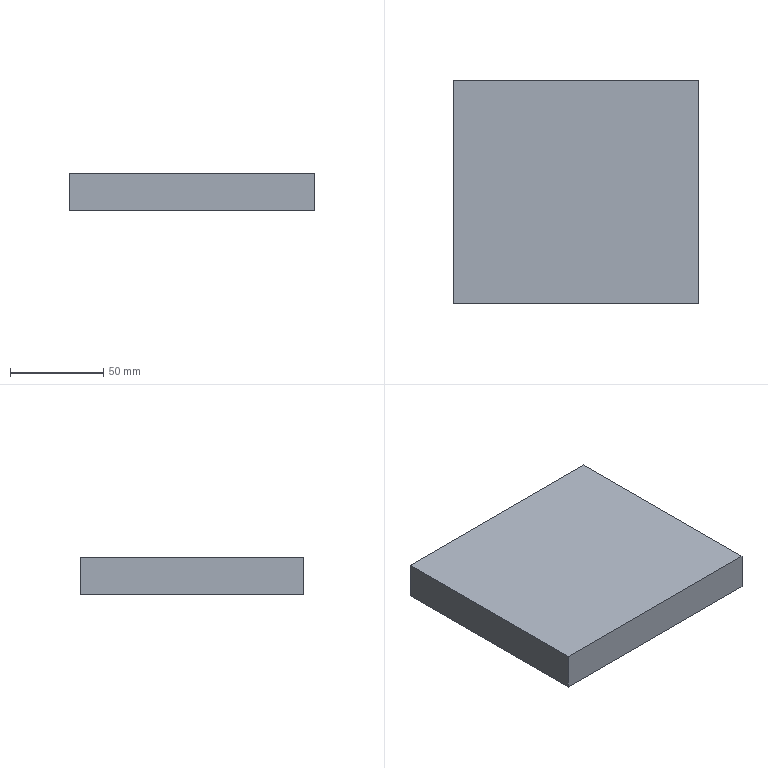Part | SolidWorks | features Extrusion 1 | 1 solid | 6 faces | box 132 x 120 x 20 mm | volume 316800 mm3 | plane 6
STEP:
#1=CARTESIAN_POINT('',(0.,120.,0.));
#2=VERTEX_POINT('',#1);
#3=CARTESIAN_POINT('',(0.,0.,0.));
#4=VERTEX_POINT('',#3);
#5=CARTESIAN_POINT('',(0.,0.,0.));
#6=DIRECTION('',(0.,-1.,0.));
#7=VECTOR('',#6,1000.);
#8=LINE('',#5,#7);
#9=EDGE_CURVE('',#2,#4,#8,.T.);
#10=ORIENTED_EDGE('',*,*,#9,.T.);
#11=CARTESIAN_POINT('',(0.,0.,20.));
#12=VERTEX_POINT('',#11);
#13=CARTESIAN_POINT('',(0.,0.,20.));
#14=DIRECTION('',(0.,0.,-1.));
#15=VECTOR('',#14,1000.);
#16=LINE('',#13,#15);
#17=EDGE_CURVE('',#12,#4,#16,.T.);
#18=ORIENTED_EDGE('',*,*,#17,.F.);
#19=CARTESIAN_POINT('',(0.,120.,20.));
#20=VERTEX_POINT('',#19);
#21=CARTESIAN_POINT('',(0.,0.,20.));
#22=DIRECTION('',(0.,-1.,0.));
#23=VECTOR('',#22,1000.);
#24=LINE('',#21,#23);
#25=EDGE_CURVE('',#20,#12,#24,.T.);
#26=ORIENTED_EDGE('',*,*,#25,.F.);
#27=CARTESIAN_POINT('',(0.,120.,20.));
#28=DIRECTION('',(0.,0.,-1.));
#29=VECTOR('',#28,1000.);
#30=LINE('',#27,#29);
#31=EDGE_CURVE('',#20,#2,#30,.T.);
#32=ORIENTED_EDGE('',*,*,#31,.T.);
#33=EDGE_LOOP('',(#10,#18,#26,#32));
#34=FACE_OUTER_BOUND('',#33,.T.);
#35=CARTESIAN_POINT('',(0.,0.,20.));
#36=DIRECTION('',(1.,0.,0.));
#37=DIRECTION('',(0.,0.,-1.));
#38=AXIS2_PLACEMENT_3D('',#35,#36,#37);
#39=PLANE('',#38);
#40=ADVANCED_FACE('',(#34),#39,.F.);
#41=CARTESIAN_POINT('',(132.,0.,0.));
#42=VERTEX_POINT('',#41);
#43=CARTESIAN_POINT('',(0.,0.,0.));
#44=DIRECTION('',(1.,0.,0.));
#45=VECTOR('',#44,1000.);
#46=LINE('',#43,#45);
#47=EDGE_CURVE('',#4,#42,#46,.T.);
#48=ORIENTED_EDGE('',*,*,#47,.T.);
#49=CARTESIAN_POINT('',(132.,0.,20.));
#50=VERTEX_POINT('',#49);
#51=CARTESIAN_POINT('',(132.,0.,20.));
#52=DIRECTION('',(0.,0.,-1.));
#53=VECTOR('',#52,1000.);
#54=LINE('',#51,#53);
#55=EDGE_CURVE('',#50,#42,#54,.T.);
#56=ORIENTED_EDGE('',*,*,#55,.F.);
#57=CARTESIAN_POINT('',(0.,0.,20.));
#58=DIRECTION('',(1.,0.,0.));
#59=VECTOR('',#58,1000.);
#60=LINE('',#57,#59);
#61=EDGE_CURVE('',#12,#50,#60,.T.);
#62=ORIENTED_EDGE('',*,*,#61,.F.);
#63=ORIENTED_EDGE('',*,*,#17,.T.);
#64=EDGE_LOOP('',(#48,#56,#62,#63));
#65=FACE_OUTER_BOUND('',#64,.T.);
#66=CARTESIAN_POINT('',(0.,0.,20.));
#67=DIRECTION('',(0.,1.,0.));
#68=DIRECTION('',(0.,0.,1.));
#69=AXIS2_PLACEMENT_3D('',#66,#67,#68);
#70=PLANE('',#69);
#71=ADVANCED_FACE('',(#65),#70,.F.);
#72=CARTESIAN_POINT('',(132.,120.,0.));
#73=VERTEX_POINT('',#72);
#74=CARTESIAN_POINT('',(132.,0.,0.));
#75=DIRECTION('',(0.,1.,0.));
#76=VECTOR('',#75,1000.);
#77=LINE('',#74,#76);
#78=EDGE_CURVE('',#42,#73,#77,.T.);
#79=ORIENTED_EDGE('',*,*,#78,.T.);
#80=CARTESIAN_POINT('',(132.,120.,20.));
#81=VERTEX_POINT('',#80);
#82=CARTESIAN_POINT('',(132.,120.,20.));
#83=DIRECTION('',(0.,0.,-1.));
#84=VECTOR('',#83,1000.);
#85=LINE('',#82,#84);
#86=EDGE_CURVE('',#81,#73,#85,.T.);
#87=ORIENTED_EDGE('',*,*,#86,.F.);
#88=CARTESIAN_POINT('',(132.,0.,20.));
#89=DIRECTION('',(0.,1.,0.));
#90=VECTOR('',#89,1000.);
#91=LINE('',#88,#90);
#92=EDGE_CURVE('',#50,#81,#91,.T.);
#93=ORIENTED_EDGE('',*,*,#92,.F.);
#94=ORIENTED_EDGE('',*,*,#55,.T.);
#95=EDGE_LOOP('',(#79,#87,#93,#94));
#96=FACE_OUTER_BOUND('',#95,.T.);
#97=CARTESIAN_POINT('',(132.,0.,20.));
#98=DIRECTION('',(-1.,0.,0.));
#99=DIRECTION('',(0.,0.,1.));
#100=AXIS2_PLACEMENT_3D('',#97,#98,#99);
#101=PLANE('',#100);
#102=ADVANCED_FACE('',(#96),#101,.F.);
#103=CARTESIAN_POINT('',(0.,120.,0.));
#104=DIRECTION('',(-1.,0.,0.));
#105=VECTOR('',#104,1000.);
#106=LINE('',#103,#105);
#107=EDGE_CURVE('',#73,#2,#106,.T.);
#108=ORIENTED_EDGE('',*,*,#107,.T.);
#109=ORIENTED_EDGE('',*,*,#31,.F.);
#110=CARTESIAN_POINT('',(0.,120.,20.));
#111=DIRECTION('',(-1.,0.,0.));
#112=VECTOR('',#111,1000.);
#113=LINE('',#110,#112);
#114=EDGE_CURVE('',#81,#20,#113,.T.);
#115=ORIENTED_EDGE('',*,*,#114,.F.);
#116=ORIENTED_EDGE('',*,*,#86,.T.);
#117=EDGE_LOOP('',(#108,#109,#115,#116));
#118=FACE_OUTER_BOUND('',#117,.T.);
#119=CARTESIAN_POINT('',(0.,120.,20.));
#120=DIRECTION('',(0.,-1.,0.));
#121=DIRECTION('',(0.,0.,-1.));
#122=AXIS2_PLACEMENT_3D('',#119,#120,#121);
#123=PLANE('',#122);
#124=ADVANCED_FACE('',(#118),#123,.F.);
#125=ORIENTED_EDGE('',*,*,#25,.T.);
#126=ORIENTED_EDGE('',*,*,#61,.T.);
#127=ORIENTED_EDGE('',*,*,#92,.T.);
#128=ORIENTED_EDGE('',*,*,#114,.T.);
#129=EDGE_LOOP('',(#125,#126,#127,#128));
#130=FACE_OUTER_BOUND('',#129,.T.);
#131=CARTESIAN_POINT('',(0.,0.,20.));
#132=DIRECTION('',(0.,0.,-1.));
#133=DIRECTION('',(-1.,0.,0.));
#134=AXIS2_PLACEMENT_3D('',#131,#132,#133);
#135=PLANE('',#134);
#136=ADVANCED_FACE('',(#130),#135,.F.);
#137=ORIENTED_EDGE('',*,*,#9,.F.);
#138=ORIENTED_EDGE('',*,*,#107,.F.);
#139=ORIENTED_EDGE('',*,*,#78,.F.);
#140=ORIENTED_EDGE('',*,*,#47,.F.);
#141=EDGE_LOOP('',(#137,#138,#139,#140));
#142=FACE_OUTER_BOUND('',#141,.T.);
#143=CARTESIAN_POINT('',(0.,0.,0.));
#144=DIRECTION('',(0.,0.,-1.));
#145=DIRECTION('',(-1.,0.,0.));
#146=AXIS2_PLACEMENT_3D('',#143,#144,#145);
#147=PLANE('',#146);
#148=ADVANCED_FACE('',(#142),#147,.T.);
#149=CLOSED_SHELL('',(#40,#71,#102,#124,#136,#148));
#150=MANIFOLD_SOLID_BREP('',#149);
#151=CARTESIAN_POINT('',(0.,0.,0.));
#152=DIRECTION('',(0.,0.,1.));
#153=DIRECTION('',(1.,0.,0.));
#154=AXIS2_PLACEMENT_3D('',#151,#152,#153);
#155=(LENGTH_UNIT()NAMED_UNIT(*)SI_UNIT(.MILLI.,.METRE.));
#156=UNCERTAINTY_MEASURE_WITH_UNIT(LENGTH_MEASURE(0.00001),#155,'','');
#157=(NAMED_UNIT(*)PLANE_ANGLE_UNIT()SI_UNIT($,.RADIAN.));
#158=(NAMED_UNIT(*)SI_UNIT($,.STERADIAN.)SOLID_ANGLE_UNIT());
#159=(GEOMETRIC_REPRESENTATION_CONTEXT(3)GLOBAL_UNCERTAINTY_ASSIGNED_CONTEXT((#156))GLOBAL_UNIT_ASSIGNED_CONTEXT((#155,#157,#158))REPRESENTATION_CONTEXT('',''));
#160=ADVANCED_BREP_SHAPE_REPRESENTATION('',(#150,#154),#159);